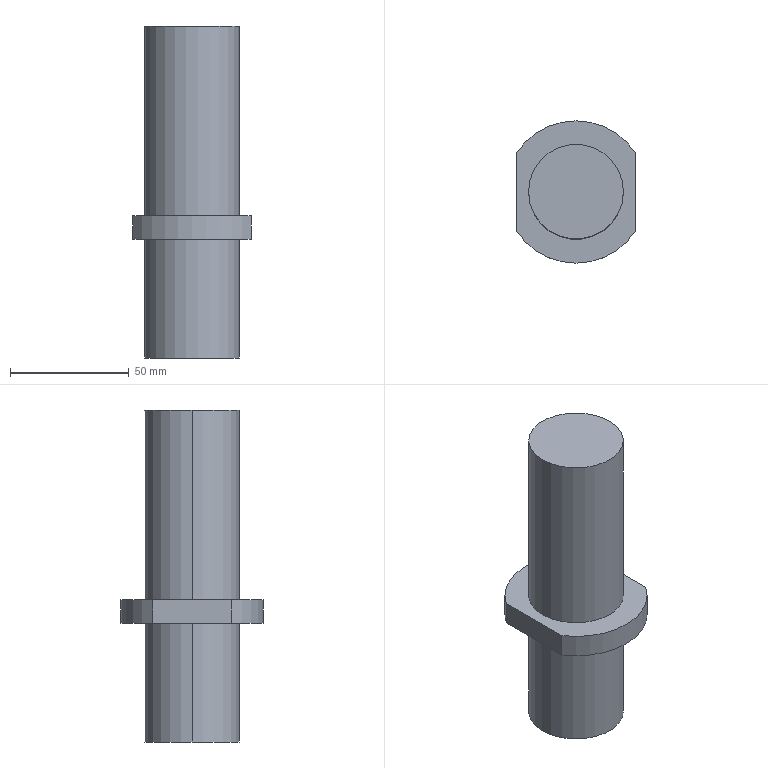Part | STEP file | Single sprocket shaft 1XG | 1 solid | 20 faces | box 50 x 60 x 140 mm | volume 188778 mm3 | cylinder 10 | plane 6 | cone 4 | commonest cylinder face diameters 5 x4 40 x4 60 x2
STEP:
#1=CARTESIAN_POINT('',(0.,0.,0.));
#2=DIRECTION('',(0.,0.,1.));
#3=DIRECTION('',(1.,0.,0.));
#4=AXIS2_PLACEMENT_3D('',#1,#2,#3);
#5=CARTESIAN_POINT('',(7.5,0.,15.));
#6=VERTEX_POINT('',#5);
#7=CARTESIAN_POINT('',(7.5,0.,0.));
#8=VERTEX_POINT('',#7);
#9=CARTESIAN_POINT('',(7.5,0.,0.));
#10=DIRECTION('',(0.,0.,-1.));
#11=VECTOR('',#10,1.);
#12=LINE('',#9,#11);
#13=CARTESIAN_POINT('',(10.,0.,0.));
#14=DIRECTION('',(0.,0.,-1.));
#15=DIRECTION('',(-1.,0.,0.));
#16=AXIS2_PLACEMENT_3D('',#13,#14,#15);
#17=CYLINDRICAL_SURFACE('',#16,2.5);
#18=CARTESIAN_POINT('',(6.283,0.));
#19=DIRECTION('',(0.,1.));
#20=VECTOR('',#19,1.);
#21=LINE('',#18,#20);
#22=(GEOMETRIC_REPRESENTATION_CONTEXT(2)PARAMETRIC_REPRESENTATION_CONTEXT()REPRESENTATION_CONTEXT('',''));
#23=DEFINITIONAL_REPRESENTATION('',(#21),#22);
#24=PCURVE('',#17,#23);
#25=CARTESIAN_POINT('',(10.,0.,0.));
#26=DIRECTION('',(0.,0.,-1.));
#27=DIRECTION('',(-1.,0.,0.));
#28=AXIS2_PLACEMENT_3D('',#25,#26,#27);
#29=CYLINDRICAL_SURFACE('',#28,2.5);
#30=CARTESIAN_POINT('',(0.,0.));
#31=DIRECTION('',(0.,1.));
#32=VECTOR('',#31,1.);
#33=LINE('',#30,#32);
#34=(GEOMETRIC_REPRESENTATION_CONTEXT(2)PARAMETRIC_REPRESENTATION_CONTEXT()REPRESENTATION_CONTEXT('',''));
#35=DEFINITIONAL_REPRESENTATION('',(#33),#34);
#36=PCURVE('',#29,#35);
#37=SURFACE_CURVE('',#12,(#24,#36),.PCURVE_S1.);
#38=EDGE_CURVE('',#6,#8,#37,.T.);
#39=ORIENTED_EDGE('',*,*,#38,.T.);
#40=CARTESIAN_POINT('',(12.5,0.,0.));
#41=VERTEX_POINT('',#40);
#42=CARTESIAN_POINT('',(10.,0.,0.));
#43=DIRECTION('',(0.,0.,-1.));
#44=DIRECTION('',(-1.,0.,0.));
#45=AXIS2_PLACEMENT_3D('',#42,#43,#44);
#46=CIRCLE('',#45,2.5);
#47=CARTESIAN_POINT('',(0.,0.));
#48=DIRECTION('',(1.,0.));
#49=VECTOR('',#48,1.);
#50=LINE('',#47,#49);
#51=(GEOMETRIC_REPRESENTATION_CONTEXT(2)PARAMETRIC_REPRESENTATION_CONTEXT()REPRESENTATION_CONTEXT('',''));
#52=DEFINITIONAL_REPRESENTATION('',(#50),#51);
#53=PCURVE('',#17,#52);
#54=CARTESIAN_POINT('',(0.,0.,0.));
#55=DIRECTION('',(0.,0.,1.));
#56=DIRECTION('',(1.,0.,0.));
#57=AXIS2_PLACEMENT_3D('',#54,#55,#56);
#58=PLANE('',#57);
#59=CARTESIAN_POINT('',(7.5,0.));
#60=CARTESIAN_POINT('',(7.5,4.33));
#61=CARTESIAN_POINT('',(11.25,2.165));
#62=CARTESIAN_POINT('',(15.,0.));
#63=CARTESIAN_POINT('',(11.25,-2.165));
#64=CARTESIAN_POINT('',(7.5,-4.33));
#65=CARTESIAN_POINT('',(7.5,0.));
#66=(BOUNDED_CURVE()B_SPLINE_CURVE(2,(#59,#60,#61,#62,#63,#64,#65),.UNSPECIFIED.,.T.,.F.)B_SPLINE_CURVE_WITH_KNOTS((1,2,2,2,2,1),(-2.094,0.,2.094,4.189,6.283,8.378),.UNSPECIFIED.)CURVE()GEOMETRIC_REPRESENTATION_ITEM()RATIONAL_B_SPLINE_CURVE((1.,0.5,1.,0.5,1.,0.5,1.))REPRESENTATION_ITEM(''));
#67=(GEOMETRIC_REPRESENTATION_CONTEXT(2)PARAMETRIC_REPRESENTATION_CONTEXT()REPRESENTATION_CONTEXT('',''));
#68=DEFINITIONAL_REPRESENTATION('',(#66),#67);
#69=PCURVE('',#58,#68);
#70=SURFACE_CURVE('',#46,(#53,#69),.PCURVE_S1.);
#71=EDGE_CURVE('',#41,#8,#70,.T.);
#72=ORIENTED_EDGE('',*,*,#71,.F.);
#73=CARTESIAN_POINT('',(12.5,0.,15.));
#74=VERTEX_POINT('',#73);
#75=CARTESIAN_POINT('',(12.5,0.,0.));
#76=DIRECTION('',(0.,0.,-1.));
#77=VECTOR('',#76,1.);
#78=LINE('',#75,#77);
#79=CARTESIAN_POINT('',(3.142,0.));
#80=DIRECTION('',(0.,1.));
#81=VECTOR('',#80,1.);
#82=LINE('',#79,#81);
#83=(GEOMETRIC_REPRESENTATION_CONTEXT(2)PARAMETRIC_REPRESENTATION_CONTEXT()REPRESENTATION_CONTEXT('',''));
#84=DEFINITIONAL_REPRESENTATION('',(#82),#83);
#85=PCURVE('',#17,#84);
#86=CARTESIAN_POINT('',(3.142,0.));
#87=DIRECTION('',(0.,1.));
#88=VECTOR('',#87,1.);
#89=LINE('',#86,#88);
#90=(GEOMETRIC_REPRESENTATION_CONTEXT(2)PARAMETRIC_REPRESENTATION_CONTEXT()REPRESENTATION_CONTEXT('',''));
#91=DEFINITIONAL_REPRESENTATION('',(#89),#90);
#92=PCURVE('',#29,#91);
#93=SURFACE_CURVE('',#78,(#85,#92),.PCURVE_S1.);
#94=EDGE_CURVE('',#74,#41,#93,.T.);
#95=ORIENTED_EDGE('',*,*,#94,.F.);
#96=CARTESIAN_POINT('',(10.,0.,15.));
#97=DIRECTION('',(0.,0.,-1.));
#98=DIRECTION('',(-1.,0.,0.));
#99=AXIS2_PLACEMENT_3D('',#96,#97,#98);
#100=CIRCLE('',#99,2.5);
#101=CARTESIAN_POINT('',(0.,-15.));
#102=DIRECTION('',(1.,0.));
#103=VECTOR('',#102,1.);
#104=LINE('',#101,#103);
#105=(GEOMETRIC_REPRESENTATION_CONTEXT(2)PARAMETRIC_REPRESENTATION_CONTEXT()REPRESENTATION_CONTEXT('',''));
#106=DEFINITIONAL_REPRESENTATION('',(#104),#105);
#107=PCURVE('',#17,#106);
#108=CARTESIAN_POINT('',(10.,0.,15.));
#109=DIRECTION('',(0.,0.,-1.));
#110=DIRECTION('',(-1.,0.,0.));
#111=AXIS2_PLACEMENT_3D('',#108,#109,#110);
#112=CONICAL_SURFACE('',#111,2.5,1.03);
#113=CARTESIAN_POINT('',(0.,0.));
#114=DIRECTION('',(1.,0.));
#115=VECTOR('',#114,1.);
#116=LINE('',#113,#115);
#117=(GEOMETRIC_REPRESENTATION_CONTEXT(2)PARAMETRIC_REPRESENTATION_CONTEXT()REPRESENTATION_CONTEXT('',''));
#118=DEFINITIONAL_REPRESENTATION('',(#116),#117);
#119=PCURVE('',#112,#118);
#120=SURFACE_CURVE('',#100,(#107,#119),.PCURVE_S1.);
#121=EDGE_CURVE('',#74,#6,#120,.T.);
#122=ORIENTED_EDGE('',*,*,#121,.T.);
#123=EDGE_LOOP('',(#39,#72,#95,#122));
#124=FACE_BOUND('',#123,.F.);
#125=ADVANCED_FACE('',(#124),#17,.F.);
#126=ORIENTED_EDGE('',*,*,#121,.F.);
#127=CARTESIAN_POINT('',(10.,0.,16.502));
#128=VERTEX_POINT('',#127);
#129=CARTESIAN_POINT('',(12.5,0.,15.));
#130=DIRECTION('',(0.8572,0.,-0.515));
#131=VECTOR('',#130,1.);
#132=LINE('',#129,#131);
#133=CARTESIAN_POINT('',(3.142,0.));
#134=DIRECTION('',(0.,1.));
#135=VECTOR('',#134,1.);
#136=LINE('',#133,#135);
#137=(GEOMETRIC_REPRESENTATION_CONTEXT(2)PARAMETRIC_REPRESENTATION_CONTEXT()REPRESENTATION_CONTEXT('',''));
#138=DEFINITIONAL_REPRESENTATION('',(#136),#137);
#139=PCURVE('',#112,#138);
#140=CARTESIAN_POINT('',(10.,0.,15.));
#141=DIRECTION('',(0.,0.,-1.));
#142=DIRECTION('',(-1.,0.,0.));
#143=AXIS2_PLACEMENT_3D('',#140,#141,#142);
#144=CONICAL_SURFACE('',#143,2.5,1.03);
#145=CARTESIAN_POINT('',(3.142,0.));
#146=DIRECTION('',(0.,1.));
#147=VECTOR('',#146,1.);
#148=LINE('',#145,#147);
#149=(GEOMETRIC_REPRESENTATION_CONTEXT(2)PARAMETRIC_REPRESENTATION_CONTEXT()REPRESENTATION_CONTEXT('',''));
#150=DEFINITIONAL_REPRESENTATION('',(#148),#149);
#151=PCURVE('',#144,#150);
#152=SURFACE_CURVE('',#132,(#139,#151),.PCURVE_S1.);
#153=EDGE_CURVE('',#128,#74,#152,.T.);
#154=ORIENTED_EDGE('',*,*,#153,.F.);
#155=CARTESIAN_POINT('',(7.5,0.,15.));
#156=DIRECTION('',(-0.8572,0.,-0.515));
#157=VECTOR('',#156,1.);
#158=LINE('',#155,#157);
#159=CARTESIAN_POINT('',(6.283,0.));
#160=DIRECTION('',(0.,1.));
#161=VECTOR('',#160,1.);
#162=LINE('',#159,#161);
#163=(GEOMETRIC_REPRESENTATION_CONTEXT(2)PARAMETRIC_REPRESENTATION_CONTEXT()REPRESENTATION_CONTEXT('',''));
#164=DEFINITIONAL_REPRESENTATION('',(#162),#163);
#165=PCURVE('',#112,#164);
#166=CARTESIAN_POINT('',(0.,0.));
#167=DIRECTION('',(0.,1.));
#168=VECTOR('',#167,1.);
#169=LINE('',#166,#168);
#170=(GEOMETRIC_REPRESENTATION_CONTEXT(2)PARAMETRIC_REPRESENTATION_CONTEXT()REPRESENTATION_CONTEXT('',''));
#171=DEFINITIONAL_REPRESENTATION('',(#169),#170);
#172=PCURVE('',#144,#171);
#173=SURFACE_CURVE('',#158,(#165,#172),.PCURVE_S1.);
#174=EDGE_CURVE('',#128,#6,#173,.T.);
#175=ORIENTED_EDGE('',*,*,#174,.T.);
#176=EDGE_LOOP('',(#126,#154,#175));
#177=FACE_BOUND('',#176,.F.);
#178=ADVANCED_FACE('',(#177),#112,.F.);
#179=CARTESIAN_POINT('',(-12.5,0.,15.));
#180=VERTEX_POINT('',#179);
#181=CARTESIAN_POINT('',(-12.5,0.,0.));
#182=VERTEX_POINT('',#181);
#183=CARTESIAN_POINT('',(-12.5,0.,0.));
#184=DIRECTION('',(0.,0.,-1.));
#185=VECTOR('',#184,1.);
#186=LINE('',#183,#185);
#187=CARTESIAN_POINT('',(-10.,0.,0.));
#188=DIRECTION('',(0.,0.,-1.));
#189=DIRECTION('',(-1.,0.,0.));
#190=AXIS2_PLACEMENT_3D('',#187,#188,#189);
#191=CYLINDRICAL_SURFACE('',#190,2.5);
#192=CARTESIAN_POINT('',(6.283,0.));
#193=DIRECTION('',(0.,1.));
#194=VECTOR('',#193,1.);
#195=LINE('',#192,#194);
#196=(GEOMETRIC_REPRESENTATION_CONTEXT(2)PARAMETRIC_REPRESENTATION_CONTEXT()REPRESENTATION_CONTEXT('',''));
#197=DEFINITIONAL_REPRESENTATION('',(#195),#196);
#198=PCURVE('',#191,#197);
#199=CARTESIAN_POINT('',(-10.,0.,0.));
#200=DIRECTION('',(0.,0.,-1.));
#201=DIRECTION('',(-1.,0.,0.));
#202=AXIS2_PLACEMENT_3D('',#199,#200,#201);
#203=CYLINDRICAL_SURFACE('',#202,2.5);
#204=CARTESIAN_POINT('',(0.,0.));
#205=DIRECTION('',(0.,1.));
#206=VECTOR('',#205,1.);
#207=LINE('',#204,#206);
#208=(GEOMETRIC_REPRESENTATION_CONTEXT(2)PARAMETRIC_REPRESENTATION_CONTEXT()REPRESENTATION_CONTEXT('',''));
#209=DEFINITIONAL_REPRESENTATION('',(#207),#208);
#210=PCURVE('',#203,#209);
#211=SURFACE_CURVE('',#186,(#198,#210),.PCURVE_S1.);
#212=EDGE_CURVE('',#180,#182,#211,.T.);
#213=ORIENTED_EDGE('',*,*,#212,.T.);
#214=CARTESIAN_POINT('',(-7.5,0.,0.));
#215=VERTEX_POINT('',#214);
#216=CARTESIAN_POINT('',(-10.,0.,0.));
#217=DIRECTION('',(0.,0.,-1.));
#218=DIRECTION('',(-1.,0.,0.));
#219=AXIS2_PLACEMENT_3D('',#216,#217,#218);
#220=CIRCLE('',#219,2.5);
#221=CARTESIAN_POINT('',(0.,0.));
#222=DIRECTION('',(1.,0.));
#223=VECTOR('',#222,1.);
#224=LINE('',#221,#223);
#225=(GEOMETRIC_REPRESENTATION_CONTEXT(2)PARAMETRIC_REPRESENTATION_CONTEXT()REPRESENTATION_CONTEXT('',''));
#226=DEFINITIONAL_REPRESENTATION('',(#224),#225);
#227=PCURVE('',#191,#226);
#228=CARTESIAN_POINT('',(-12.5,0.));
#229=CARTESIAN_POINT('',(-12.5,4.33));
#230=CARTESIAN_POINT('',(-8.75,2.165));
#231=CARTESIAN_POINT('',(-5.,0.));
#232=CARTESIAN_POINT('',(-8.75,-2.165));
#233=CARTESIAN_POINT('',(-12.5,-4.33));
#234=CARTESIAN_POINT('',(-12.5,0.));
#235=(BOUNDED_CURVE()B_SPLINE_CURVE(2,(#228,#229,#230,#231,#232,#233,#234),.UNSPECIFIED.,.T.,.F.)B_SPLINE_CURVE_WITH_KNOTS((1,2,2,2,2,1),(-2.094,0.,2.094,4.189,6.283,8.378),.UNSPECIFIED.)CURVE()GEOMETRIC_REPRESENTATION_ITEM()RATIONAL_B_SPLINE_CURVE((1.,0.5,1.,0.5,1.,0.5,1.))REPRESENTATION_ITEM(''));
#236=(GEOMETRIC_REPRESENTATION_CONTEXT(2)PARAMETRIC_REPRESENTATION_CONTEXT()REPRESENTATION_CONTEXT('',''));
#237=DEFINITIONAL_REPRESENTATION('',(#235),#236);
#238=PCURVE('',#58,#237);
#239=SURFACE_CURVE('',#220,(#227,#238),.PCURVE_S1.);
#240=EDGE_CURVE('',#215,#182,#239,.T.);
#241=ORIENTED_EDGE('',*,*,#240,.F.);
#242=CARTESIAN_POINT('',(-7.5,0.,15.));
#243=VERTEX_POINT('',#242);
#244=CARTESIAN_POINT('',(-7.5,0.,0.));
#245=DIRECTION('',(0.,0.,-1.));
#246=VECTOR('',#245,1.);
#247=LINE('',#244,#246);
#248=CARTESIAN_POINT('',(3.142,0.));
#249=DIRECTION('',(0.,1.));
#250=VECTOR('',#249,1.);
#251=LINE('',#248,#250);
#252=(GEOMETRIC_REPRESENTATION_CONTEXT(2)PARAMETRIC_REPRESENTATION_CONTEXT()REPRESENTATION_CONTEXT('',''));
#253=DEFINITIONAL_REPRESENTATION('',(#251),#252);
#254=PCURVE('',#191,#253);
#255=CARTESIAN_POINT('',(3.142,0.));
#256=DIRECTION('',(0.,1.));
#257=VECTOR('',#256,1.);
#258=LINE('',#255,#257);
#259=(GEOMETRIC_REPRESENTATION_CONTEXT(2)PARAMETRIC_REPRESENTATION_CONTEXT()REPRESENTATION_CONTEXT('',''));
#260=DEFINITIONAL_REPRESENTATION('',(#258),#259);
#261=PCURVE('',#203,#260);
#262=SURFACE_CURVE('',#247,(#254,#261),.PCURVE_S1.);
#263=EDGE_CURVE('',#243,#215,#262,.T.);
#264=ORIENTED_EDGE('',*,*,#263,.F.);
#265=CARTESIAN_POINT('',(-10.,0.,15.));
#266=DIRECTION('',(0.,0.,-1.));
#267=DIRECTION('',(-1.,0.,0.));
#268=AXIS2_PLACEMENT_3D('',#265,#266,#267);
#269=CIRCLE('',#268,2.5);
#270=CARTESIAN_POINT('',(0.,-15.));
#271=DIRECTION('',(1.,0.));
#272=VECTOR('',#271,1.);
#273=LINE('',#270,#272);
#274=(GEOMETRIC_REPRESENTATION_CONTEXT(2)PARAMETRIC_REPRESENTATION_CONTEXT()REPRESENTATION_CONTEXT('',''));
#275=DEFINITIONAL_REPRESENTATION('',(#273),#274);
#276=PCURVE('',#191,#275);
#277=CARTESIAN_POINT('',(-10.,0.,15.));
#278=DIRECTION('',(0.,0.,-1.));
#279=DIRECTION('',(-1.,0.,0.));
#280=AXIS2_PLACEMENT_3D('',#277,#278,#279);
#281=CONICAL_SURFACE('',#280,2.5,1.03);
#282=CARTESIAN_POINT('',(0.,0.));
#283=DIRECTION('',(1.,0.));
#284=VECTOR('',#283,1.);
#285=LINE('',#282,#284);
#286=(GEOMETRIC_REPRESENTATION_CONTEXT(2)PARAMETRIC_REPRESENTATION_CONTEXT()REPRESENTATION_CONTEXT('',''));
#287=DEFINITIONAL_REPRESENTATION('',(#285),#286);
#288=PCURVE('',#281,#287);
#289=SURFACE_CURVE('',#269,(#276,#288),.PCURVE_S1.);
#290=EDGE_CURVE('',#243,#180,#289,.T.);
#291=ORIENTED_EDGE('',*,*,#290,.T.);
#292=EDGE_LOOP('',(#213,#241,#264,#291));
#293=FACE_BOUND('',#292,.F.);
#294=ADVANCED_FACE('',(#293),#191,.F.);
#295=ORIENTED_EDGE('',*,*,#290,.F.);
#296=CARTESIAN_POINT('',(-10.,0.,16.502));
#297=VERTEX_POINT('',#296);
#298=CARTESIAN_POINT('',(-7.5,0.,15.));
#299=DIRECTION('',(0.8572,0.,-0.515));
#300=VECTOR('',#299,1.);
#301=LINE('',#298,#300);
#302=CARTESIAN_POINT('',(3.142,0.));
#303=DIRECTION('',(0.,1.));
#304=VECTOR('',#303,1.);
#305=LINE('',#302,#304);
#306=(GEOMETRIC_REPRESENTATION_CONTEXT(2)PARAMETRIC_REPRESENTATION_CONTEXT()REPRESENTATION_CONTEXT('',''));
#307=DEFINITIONAL_REPRESENTATION('',(#305),#306);
#308=PCURVE('',#281,#307);
#309=CARTESIAN_POINT('',(-10.,0.,15.));
#310=DIRECTION('',(0.,0.,-1.));
#311=DIRECTION('',(-1.,0.,0.));
#312=AXIS2_PLACEMENT_3D('',#309,#310,#311);
#313=CONICAL_SURFACE('',#312,2.5,1.03);
#314=CARTESIAN_POINT('',(3.142,0.));
#315=DIRECTION('',(0.,1.));
#316=VECTOR('',#315,1.);
#317=LINE('',#314,#316);
#318=(GEOMETRIC_REPRESENTATION_CONTEXT(2)PARAMETRIC_REPRESENTATION_CONTEXT()REPRESENTATION_CONTEXT('',''));
#319=DEFINITIONAL_REPRESENTATION('',(#317),#318);
#320=PCURVE('',#313,#319);
#321=SURFACE_CURVE('',#301,(#308,#320),.PCURVE_S1.);
#322=EDGE_CURVE('',#297,#243,#321,.T.);
#323=ORIENTED_EDGE('',*,*,#322,.F.);
#324=CARTESIAN_POINT('',(-12.5,0.,15.));
#325=DIRECTION('',(-0.8572,0.,-0.515));
#326=VECTOR('',#325,1.);
#327=LINE('',#324,#326);
#328=CARTESIAN_POINT('',(6.283,0.));
#329=DIRECTION('',(0.,1.));
#330=VECTOR('',#329,1.);
#331=LINE('',#328,#330);
#332=(GEOMETRIC_REPRESENTATION_CONTEXT(2)PARAMETRIC_REPRESENTATION_CONTEXT()REPRESENTATION_CONTEXT('',''));
#333=DEFINITIONAL_REPRESENTATION('',(#331),#332);
#334=PCURVE('',#281,#333);
#335=CARTESIAN_POINT('',(0.,0.));
#336=DIRECTION('',(0.,1.));
#337=VECTOR('',#336,1.);
#338=LINE('',#335,#337);
#339=(GEOMETRIC_REPRESENTATION_CONTEXT(2)PARAMETRIC_REPRESENTATION_CONTEXT()REPRESENTATION_CONTEXT('',''));
#340=DEFINITIONAL_REPRESENTATION('',(#338),#339);
#341=PCURVE('',#313,#340);
#342=SURFACE_CURVE('',#327,(#334,#341),.PCURVE_S1.);
#343=EDGE_CURVE('',#297,#180,#342,.T.);
#344=ORIENTED_EDGE('',*,*,#343,.T.);
#345=EDGE_LOOP('',(#295,#323,#344));
#346=FACE_BOUND('',#345,.F.);
#347=ADVANCED_FACE('',(#346),#281,.F.);
#348=CARTESIAN_POINT('',(20.,0.,140.));
#349=VERTEX_POINT('',#348);
#350=CARTESIAN_POINT('',(-20.,0.,140.));
#351=VERTEX_POINT('',#350);
#352=CARTESIAN_POINT('',(0.,0.,140.));
#353=DIRECTION('',(0.,0.,1.));
#354=DIRECTION('',(1.,0.,0.));
#355=AXIS2_PLACEMENT_3D('',#352,#353,#354);
#356=CIRCLE('',#355,20.);
#357=CARTESIAN_POINT('',(0.,0.,140.));
#358=DIRECTION('',(0.,0.,-1.));
#359=DIRECTION('',(-1.,0.,0.));
#360=AXIS2_PLACEMENT_3D('',#357,#358,#359);
#361=CYLINDRICAL_SURFACE('',#360,20.);
#362=CARTESIAN_POINT('',(3.142,0.));
#363=DIRECTION('',(-1.,0.));
#364=VECTOR('',#363,1.);
#365=LINE('',#362,#364);
#366=(GEOMETRIC_REPRESENTATION_CONTEXT(2)PARAMETRIC_REPRESENTATION_CONTEXT()REPRESENTATION_CONTEXT('',''));
#367=DEFINITIONAL_REPRESENTATION('',(#365),#366);
#368=PCURVE('',#361,#367);
#369=CARTESIAN_POINT('',(0.,0.,140.));
#370=DIRECTION('',(0.,0.,1.));
#371=DIRECTION('',(1.,0.,0.));
#372=AXIS2_PLACEMENT_3D('',#369,#370,#371);
#373=PLANE('',#372);
#374=CARTESIAN_POINT('',(0.,0.));
#375=DIRECTION('',(1.,0.));
#376=AXIS2_PLACEMENT_2D('',#374,#375);
#377=CIRCLE('',#376,20.);
#378=(GEOMETRIC_REPRESENTATION_CONTEXT(2)PARAMETRIC_REPRESENTATION_CONTEXT()REPRESENTATION_CONTEXT('',''));
#379=DEFINITIONAL_REPRESENTATION('',(#377),#378);
#380=PCURVE('',#373,#379);
#381=SURFACE_CURVE('',#356,(#368,#380),.PCURVE_S1.);
#382=EDGE_CURVE('',#349,#351,#381,.T.);
#383=ORIENTED_EDGE('',*,*,#382,.F.);
#384=CARTESIAN_POINT('',(20.,0.,60.));
#385=VERTEX_POINT('',#384);
#386=CARTESIAN_POINT('',(20.,0.,140.));
#387=DIRECTION('',(0.,0.,-1.));
#388=VECTOR('',#387,1.);
#389=LINE('',#386,#388);
#390=CARTESIAN_POINT('',(3.142,0.));
#391=DIRECTION('',(0.,1.));
#392=VECTOR('',#391,1.);
#393=LINE('',#390,#392);
#394=(GEOMETRIC_REPRESENTATION_CONTEXT(2)PARAMETRIC_REPRESENTATION_CONTEXT()REPRESENTATION_CONTEXT('',''));
#395=DEFINITIONAL_REPRESENTATION('',(#393),#394);
#396=PCURVE('',#361,#395);
#397=CARTESIAN_POINT('',(0.,0.,140.));
#398=DIRECTION('',(0.,0.,-1.));
#399=DIRECTION('',(-1.,0.,0.));
#400=AXIS2_PLACEMENT_3D('',#397,#398,#399);
#401=CYLINDRICAL_SURFACE('',#400,20.);
#402=CARTESIAN_POINT('',(3.142,0.));
#403=DIRECTION('',(0.,1.));
#404=VECTOR('',#403,1.);
#405=LINE('',#402,#404);
#406=(GEOMETRIC_REPRESENTATION_CONTEXT(2)PARAMETRIC_REPRESENTATION_CONTEXT()REPRESENTATION_CONTEXT('',''));
#407=DEFINITIONAL_REPRESENTATION('',(#405),#406);
#408=PCURVE('',#401,#407);
#409=SURFACE_CURVE('',#389,(#396,#408),.PCURVE_S1.);
#410=EDGE_CURVE('',#349,#385,#409,.T.);
#411=ORIENTED_EDGE('',*,*,#410,.T.);
#412=CARTESIAN_POINT('',(-20.,0.,60.));
#413=VERTEX_POINT('',#412);
#414=CARTESIAN_POINT('',(0.,0.,60.));
#415=DIRECTION('',(0.,0.,1.));
#416=DIRECTION('',(1.,0.,0.));
#417=AXIS2_PLACEMENT_3D('',#414,#415,#416);
#418=CIRCLE('',#417,20.);
#419=CARTESIAN_POINT('',(3.142,80.));
#420=DIRECTION('',(-1.,0.));
#421=VECTOR('',#420,1.);
#422=LINE('',#419,#421);
#423=(GEOMETRIC_REPRESENTATION_CONTEXT(2)PARAMETRIC_REPRESENTATION_CONTEXT()REPRESENTATION_CONTEXT('',''));
#424=DEFINITIONAL_REPRESENTATION('',(#422),#423);
#425=PCURVE('',#361,#424);
#426=CARTESIAN_POINT('',(0.,0.,60.));
#427=DIRECTION('',(0.,0.,1.));
#428=DIRECTION('',(1.,0.,0.));
#429=AXIS2_PLACEMENT_3D('',#426,#427,#428);
#430=PLANE('',#429);
#431=CARTESIAN_POINT('',(0.,0.));
#432=DIRECTION('',(1.,0.));
#433=AXIS2_PLACEMENT_2D('',#431,#432);
#434=CIRCLE('',#433,20.);
#435=(GEOMETRIC_REPRESENTATION_CONTEXT(2)PARAMETRIC_REPRESENTATION_CONTEXT()REPRESENTATION_CONTEXT('',''));
#436=DEFINITIONAL_REPRESENTATION('',(#434),#435);
#437=PCURVE('',#430,#436);
#438=SURFACE_CURVE('',#418,(#425,#437),.PCURVE_S1.);
#439=EDGE_CURVE('',#385,#413,#438,.T.);
#440=ORIENTED_EDGE('',*,*,#439,.T.);
#441=CARTESIAN_POINT('',(-20.,0.,140.));
#442=DIRECTION('',(0.,0.,-1.));
#443=VECTOR('',#442,1.);
#444=LINE('',#441,#443);
#445=CARTESIAN_POINT('',(0.,0.));
#446=DIRECTION('',(0.,1.));
#447=VECTOR('',#446,1.);
#448=LINE('',#445,#447);
#449=(GEOMETRIC_REPRESENTATION_CONTEXT(2)PARAMETRIC_REPRESENTATION_CONTEXT()REPRESENTATION_CONTEXT('',''));
#450=DEFINITIONAL_REPRESENTATION('',(#448),#449);
#451=PCURVE('',#361,#450);
#452=CARTESIAN_POINT('',(6.283,0.));
#453=DIRECTION('',(0.,1.));
#454=VECTOR('',#453,1.);
#455=LINE('',#452,#454);
#456=(GEOMETRIC_REPRESENTATION_CONTEXT(2)PARAMETRIC_REPRESENTATION_CONTEXT()REPRESENTATION_CONTEXT('',''));
#457=DEFINITIONAL_REPRESENTATION('',(#455),#456);
#458=PCURVE('',#401,#457);
#459=SURFACE_CURVE('',#444,(#451,#458),.PCURVE_S1.);
#460=EDGE_CURVE('',#351,#413,#459,.T.);
#461=ORIENTED_EDGE('',*,*,#460,.F.);
#462=EDGE_LOOP('',(#383,#411,#440,#461));
#463=FACE_BOUND('',#462,.T.);
#464=ADVANCED_FACE('',(#463),#361,.T.);
#465=CARTESIAN_POINT('',(20.,0.,50.));
#466=VERTEX_POINT('',#465);
#467=CARTESIAN_POINT('',(-20.,0.,50.));
#468=VERTEX_POINT('',#467);
#469=CARTESIAN_POINT('',(0.,0.,50.));
#470=DIRECTION('',(0.,0.,1.));
#471=DIRECTION('',(1.,0.,0.));
#472=AXIS2_PLACEMENT_3D('',#469,#470,#471);
#473=CIRCLE('',#472,20.);
#474=CARTESIAN_POINT('',(0.,0.,50.));
#475=DIRECTION('',(0.,0.,-1.));
#476=DIRECTION('',(-1.,0.,0.));
#477=AXIS2_PLACEMENT_3D('',#474,#475,#476);
#478=CYLINDRICAL_SURFACE('',#477,20.);
#479=CARTESIAN_POINT('',(3.142,0.));
#480=DIRECTION('',(-1.,0.));
#481=VECTOR('',#480,1.);
#482=LINE('',#479,#481);
#483=(GEOMETRIC_REPRESENTATION_CONTEXT(2)PARAMETRIC_REPRESENTATION_CONTEXT()REPRESENTATION_CONTEXT('',''));
#484=DEFINITIONAL_REPRESENTATION('',(#482),#483);
#485=PCURVE('',#478,#484);
#486=CARTESIAN_POINT('',(0.,0.,50.));
#487=DIRECTION('',(0.,0.,1.));
#488=DIRECTION('',(1.,0.,0.));
#489=AXIS2_PLACEMENT_3D('',#486,#487,#488);
#490=PLANE('',#489);
#491=CARTESIAN_POINT('',(0.,0.));
#492=DIRECTION('',(1.,0.));
#493=AXIS2_PLACEMENT_2D('',#491,#492);
#494=CIRCLE('',#493,20.);
#495=(GEOMETRIC_REPRESENTATION_CONTEXT(2)PARAMETRIC_REPRESENTATION_CONTEXT()REPRESENTATION_CONTEXT('',''));
#496=DEFINITIONAL_REPRESENTATION('',(#494),#495);
#497=PCURVE('',#490,#496);
#498=SURFACE_CURVE('',#473,(#485,#497),.PCURVE_S1.);
#499=EDGE_CURVE('',#466,#468,#498,.T.);
#500=ORIENTED_EDGE('',*,*,#499,.F.);
#501=CARTESIAN_POINT('',(20.,0.,0.));
#502=VERTEX_POINT('',#501);
#503=CARTESIAN_POINT('',(20.,0.,50.));
#504=DIRECTION('',(0.,0.,-1.));
#505=VECTOR('',#504,1.);
#506=LINE('',#503,#505);
#507=CARTESIAN_POINT('',(3.142,0.));
#508=DIRECTION('',(0.,1.));
#509=VECTOR('',#508,1.);
#510=LINE('',#507,#509);
#511=(GEOMETRIC_REPRESENTATION_CONTEXT(2)PARAMETRIC_REPRESENTATION_CONTEXT()REPRESENTATION_CONTEXT('',''));
#512=DEFINITIONAL_REPRESENTATION('',(#510),#511);
#513=PCURVE('',#478,#512);
#514=CARTESIAN_POINT('',(0.,0.,50.));
#515=DIRECTION('',(0.,0.,-1.));
#516=DIRECTION('',(-1.,0.,0.));
#517=AXIS2_PLACEMENT_3D('',#514,#515,#516);
#518=CYLINDRICAL_SURFACE('',#517,20.);
#519=CARTESIAN_POINT('',(3.142,0.));
#520=DIRECTION('',(0.,1.));
#521=VECTOR('',#520,1.);
#522=LINE('',#519,#521);
#523=(GEOMETRIC_REPRESENTATION_CONTEXT(2)PARAMETRIC_REPRESENTATION_CONTEXT()REPRESENTATION_CONTEXT('',''));
#524=DEFINITIONAL_REPRESENTATION('',(#522),#523);
#525=PCURVE('',#518,#524);
#526=SURFACE_CURVE('',#506,(#513,#525),.PCURVE_S1.);
#527=EDGE_CURVE('',#466,#502,#526,.T.);
#528=ORIENTED_EDGE('',*,*,#527,.T.);
#529=CARTESIAN_POINT('',(-20.,0.,0.));
#530=VERTEX_POINT('',#529);
#531=CARTESIAN_POINT('',(0.,0.,0.));
#532=DIRECTION('',(0.,0.,1.));
#533=DIRECTION('',(1.,0.,0.));
#534=AXIS2_PLACEMENT_3D('',#531,#532,#533);
#535=CIRCLE('',#534,20.);
#536=CARTESIAN_POINT('',(3.142,50.));
#537=DIRECTION('',(-1.,0.));
#538=VECTOR('',#537,1.);
#539=LINE('',#536,#538);
#540=(GEOMETRIC_REPRESENTATION_CONTEXT(2)PARAMETRIC_REPRESENTATION_CONTEXT()REPRESENTATION_CONTEXT('',''));
#541=DEFINITIONAL_REPRESENTATION('',(#539),#540);
#542=PCURVE('',#478,#541);
#543=CARTESIAN_POINT('',(0.,0.));
#544=DIRECTION('',(1.,0.));
#545=AXIS2_PLACEMENT_2D('',#543,#544);
#546=CIRCLE('',#545,20.);
#547=(GEOMETRIC_REPRESENTATION_CONTEXT(2)PARAMETRIC_REPRESENTATION_CONTEXT()REPRESENTATION_CONTEXT('',''));
#548=DEFINITIONAL_REPRESENTATION('',(#546),#547);
#549=PCURVE('',#58,#548);
#550=SURFACE_CURVE('',#535,(#542,#549),.PCURVE_S1.);
#551=EDGE_CURVE('',#502,#530,#550,.T.);
#552=ORIENTED_EDGE('',*,*,#551,.T.);
#553=CARTESIAN_POINT('',(-20.,0.,50.));
#554=DIRECTION('',(0.,0.,-1.));
#555=VECTOR('',#554,1.);
#556=LINE('',#553,#555);
#557=CARTESIAN_POINT('',(0.,0.));
#558=DIRECTION('',(0.,1.));
#559=VECTOR('',#558,1.);
#560=LINE('',#557,#559);
#561=(GEOMETRIC_REPRESENTATION_CONTEXT(2)PARAMETRIC_REPRESENTATION_CONTEXT()REPRESENTATION_CONTEXT('',''));
#562=DEFINITIONAL_REPRESENTATION('',(#560),#561);
#563=PCURVE('',#478,#562);
#564=CARTESIAN_POINT('',(6.283,0.));
#565=DIRECTION('',(0.,1.));
#566=VECTOR('',#565,1.);
#567=LINE('',#564,#566);
#568=(GEOMETRIC_REPRESENTATION_CONTEXT(2)PARAMETRIC_REPRESENTATION_CONTEXT()REPRESENTATION_CONTEXT('',''));
#569=DEFINITIONAL_REPRESENTATION('',(#567),#568);
#570=PCURVE('',#518,#569);
#571=SURFACE_CURVE('',#556,(#563,#570),.PCURVE_S1.);
#572=EDGE_CURVE('',#468,#530,#571,.T.);
#573=ORIENTED_EDGE('',*,*,#572,.F.);
#574=EDGE_LOOP('',(#500,#528,#552,#573));
#575=FACE_BOUND('',#574,.T.);
#576=ADVANCED_FACE('',(#575),#478,.T.);
#577=CARTESIAN_POINT('',(-25.,-16.583,60.));
#578=VERTEX_POINT('',#577);
#579=CARTESIAN_POINT('',(25.,-16.583,60.));
#580=VERTEX_POINT('',#579);
#581=CARTESIAN_POINT('',(0.,0.,60.));
#582=DIRECTION('',(0.,0.,1.));
#583=DIRECTION('',(1.,0.,0.));
#584=AXIS2_PLACEMENT_3D('',#581,#582,#583);
#585=CIRCLE('',#584,30.);
#586=CARTESIAN_POINT('',(0.,0.));
#587=DIRECTION('',(1.,0.));
#588=AXIS2_PLACEMENT_2D('',#586,#587);
#589=CIRCLE('',#588,30.);
#590=(GEOMETRIC_REPRESENTATION_CONTEXT(2)PARAMETRIC_REPRESENTATION_CONTEXT()REPRESENTATION_CONTEXT('',''));
#591=DEFINITIONAL_REPRESENTATION('',(#589),#590);
#592=PCURVE('',#430,#591);
#593=CARTESIAN_POINT('',(0.,0.,60.));
#594=DIRECTION('',(0.,0.,-1.));
#595=DIRECTION('',(-1.,0.,0.));
#596=AXIS2_PLACEMENT_3D('',#593,#594,#595);
#597=CYLINDRICAL_SURFACE('',#596,30.);
#598=CARTESIAN_POINT('',(9.425,0.));
#599=DIRECTION('',(-1.,0.));
#600=VECTOR('',#599,1.);
#601=LINE('',#598,#600);
#602=(GEOMETRIC_REPRESENTATION_CONTEXT(2)PARAMETRIC_REPRESENTATION_CONTEXT()REPRESENTATION_CONTEXT('',''));
#603=DEFINITIONAL_REPRESENTATION('',(#601),#602);
#604=PCURVE('',#597,#603);
#605=SURFACE_CURVE('',#585,(#592,#604),.PCURVE_S1.);
#606=EDGE_CURVE('',#578,#580,#605,.T.);
#607=ORIENTED_EDGE('',*,*,#606,.T.);
#608=CARTESIAN_POINT('',(25.,16.583,60.));
#609=VERTEX_POINT('',#608);
#610=CARTESIAN_POINT('',(25.,16.583,60.));
#611=DIRECTION('',(0.,1.,0.));
#612=VECTOR('',#611,1.);
#613=LINE('',#610,#612);
#614=CARTESIAN_POINT('',(25.,16.583));
#615=DIRECTION('',(0.,1.));
#616=VECTOR('',#615,1.);
#617=LINE('',#614,#616);
#618=(GEOMETRIC_REPRESENTATION_CONTEXT(2)PARAMETRIC_REPRESENTATION_CONTEXT()REPRESENTATION_CONTEXT('',''));
#619=DEFINITIONAL_REPRESENTATION('',(#617),#618);
#620=PCURVE('',#430,#619);
#621=CARTESIAN_POINT('',(25.,16.583,60.));
#622=DIRECTION('',(-1.,0.,0.));
#623=DIRECTION('',(0.,0.,1.));
#624=AXIS2_PLACEMENT_3D('',#621,#622,#623);
#625=PLANE('',#624);
#626=CARTESIAN_POINT('',(0.,0.));
#627=DIRECTION('',(0.,1.));
#628=VECTOR('',#627,1.);
#629=LINE('',#626,#628);
#630=(GEOMETRIC_REPRESENTATION_CONTEXT(2)PARAMETRIC_REPRESENTATION_CONTEXT()REPRESENTATION_CONTEXT('',''));
#631=DEFINITIONAL_REPRESENTATION('',(#629),#630);
#632=PCURVE('',#625,#631);
#633=SURFACE_CURVE('',#613,(#620,#632),.PCURVE_S1.);
#634=EDGE_CURVE('',#580,#609,#633,.T.);
#635=ORIENTED_EDGE('',*,*,#634,.T.);
#636=CARTESIAN_POINT('',(-25.,16.583,60.));
#637=VERTEX_POINT('',#636);
#638=CARTESIAN_POINT('',(0.,0.,60.));
#639=DIRECTION('',(0.,0.,1.));
#640=DIRECTION('',(1.,0.,0.));
#641=AXIS2_PLACEMENT_3D('',#638,#639,#640);
#642=CIRCLE('',#641,30.);
#643=CARTESIAN_POINT('',(0.,0.));
#644=DIRECTION('',(1.,0.));
#645=AXIS2_PLACEMENT_2D('',#643,#644);
#646=CIRCLE('',#645,30.);
#647=(GEOMETRIC_REPRESENTATION_CONTEXT(2)PARAMETRIC_REPRESENTATION_CONTEXT()REPRESENTATION_CONTEXT('',''));
#648=DEFINITIONAL_REPRESENTATION('',(#646),#647);
#649=PCURVE('',#430,#648);
#650=CARTESIAN_POINT('',(0.,0.,60.));
#651=DIRECTION('',(0.,0.,-1.));
#652=DIRECTION('',(-1.,0.,0.));
#653=AXIS2_PLACEMENT_3D('',#650,#651,#652);
#654=CYLINDRICAL_SURFACE('',#653,30.);
#655=CARTESIAN_POINT('',(3.142,0.));
#656=DIRECTION('',(-1.,0.));
#657=VECTOR('',#656,1.);
#658=LINE('',#655,#657);
#659=(GEOMETRIC_REPRESENTATION_CONTEXT(2)PARAMETRIC_REPRESENTATION_CONTEXT()REPRESENTATION_CONTEXT('',''));
#660=DEFINITIONAL_REPRESENTATION('',(#658),#659);
#661=PCURVE('',#654,#660);
#662=SURFACE_CURVE('',#642,(#649,#661),.PCURVE_S1.);
#663=EDGE_CURVE('',#609,#637,#662,.T.);
#664=ORIENTED_EDGE('',*,*,#663,.T.);
#665=CARTESIAN_POINT('',(-25.,16.583,60.));
#666=DIRECTION('',(0.,-1.,0.));
#667=VECTOR('',#666,1.);
#668=LINE('',#665,#667);
#669=CARTESIAN_POINT('',(-25.,16.583));
#670=DIRECTION('',(0.,-1.));
#671=VECTOR('',#670,1.);
#672=LINE('',#669,#671);
#673=(GEOMETRIC_REPRESENTATION_CONTEXT(2)PARAMETRIC_REPRESENTATION_CONTEXT()REPRESENTATION_CONTEXT('',''));
#674=DEFINITIONAL_REPRESENTATION('',(#672),#673);
#675=PCURVE('',#430,#674);
#676=CARTESIAN_POINT('',(-25.,16.583,60.));
#677=DIRECTION('',(1.,0.,0.));
#678=DIRECTION('',(0.,0.,-1.));
#679=AXIS2_PLACEMENT_3D('',#676,#677,#678);
#680=PLANE('',#679);
#681=CARTESIAN_POINT('',(0.,0.));
#682=DIRECTION('',(0.,-1.));
#683=VECTOR('',#682,1.);
#684=LINE('',#681,#683);
#685=(GEOMETRIC_REPRESENTATION_CONTEXT(2)PARAMETRIC_REPRESENTATION_CONTEXT()REPRESENTATION_CONTEXT('',''));
#686=DEFINITIONAL_REPRESENTATION('',(#684),#685);
#687=PCURVE('',#680,#686);
#688=SURFACE_CURVE('',#668,(#675,#687),.PCURVE_S1.);
#689=EDGE_CURVE('',#637,#578,#688,.T.);
#690=ORIENTED_EDGE('',*,*,#689,.T.);
#691=EDGE_LOOP('',(#607,#635,#664,#690));
#692=FACE_BOUND('',#691,.T.);
#693=CARTESIAN_POINT('',(0.,0.,60.));
#694=DIRECTION('',(0.,0.,1.));
#695=DIRECTION('',(1.,0.,0.));
#696=AXIS2_PLACEMENT_3D('',#693,#694,#695);
#697=CIRCLE('',#696,20.);
#698=CARTESIAN_POINT('',(0.,0.));
#699=DIRECTION('',(1.,0.));
#700=AXIS2_PLACEMENT_2D('',#698,#699);
#701=CIRCLE('',#700,20.);
#702=(GEOMETRIC_REPRESENTATION_CONTEXT(2)PARAMETRIC_REPRESENTATION_CONTEXT()REPRESENTATION_CONTEXT('',''));
#703=DEFINITIONAL_REPRESENTATION('',(#701),#702);
#704=PCURVE('',#430,#703);
#705=CARTESIAN_POINT('',(9.425,80.));
#706=DIRECTION('',(-1.,0.));
#707=VECTOR('',#706,1.);
#708=LINE('',#705,#707);
#709=(GEOMETRIC_REPRESENTATION_CONTEXT(2)PARAMETRIC_REPRESENTATION_CONTEXT()REPRESENTATION_CONTEXT('',''));
#710=DEFINITIONAL_REPRESENTATION('',(#708),#709);
#711=PCURVE('',#401,#710);
#712=SURFACE_CURVE('',#697,(#704,#711),.PCURVE_S1.);
#713=EDGE_CURVE('',#413,#385,#712,.T.);
#714=ORIENTED_EDGE('',*,*,#713,.F.);
#715=ORIENTED_EDGE('',*,*,#439,.F.);
#716=EDGE_LOOP('',(#714,#715));
#717=FACE_BOUND('',#716,.T.);
#718=ADVANCED_FACE('',(#692,#717),#430,.T.);
#719=ORIENTED_EDGE('',*,*,#527,.F.);
#720=CARTESIAN_POINT('',(0.,0.,50.));
#721=DIRECTION('',(0.,0.,1.));
#722=DIRECTION('',(1.,0.,0.));
#723=AXIS2_PLACEMENT_3D('',#720,#721,#722);
#724=CIRCLE('',#723,20.);
#725=CARTESIAN_POINT('',(9.425,0.));
#726=DIRECTION('',(-1.,0.));
#727=VECTOR('',#726,1.);
#728=LINE('',#725,#727);
#729=(GEOMETRIC_REPRESENTATION_CONTEXT(2)PARAMETRIC_REPRESENTATION_CONTEXT()REPRESENTATION_CONTEXT('',''));
#730=DEFINITIONAL_REPRESENTATION('',(#728),#729);
#731=PCURVE('',#518,#730);
#732=CARTESIAN_POINT('',(0.,0.));
#733=DIRECTION('',(1.,0.));
#734=AXIS2_PLACEMENT_2D('',#732,#733);
#735=CIRCLE('',#734,20.);
#736=(GEOMETRIC_REPRESENTATION_CONTEXT(2)PARAMETRIC_REPRESENTATION_CONTEXT()REPRESENTATION_CONTEXT('',''));
#737=DEFINITIONAL_REPRESENTATION('',(#735),#736);
#738=PCURVE('',#490,#737);
#739=SURFACE_CURVE('',#724,(#731,#738),.PCURVE_S1.);
#740=EDGE_CURVE('',#468,#466,#739,.T.);
#741=ORIENTED_EDGE('',*,*,#740,.F.);
#742=ORIENTED_EDGE('',*,*,#572,.T.);
#743=CARTESIAN_POINT('',(0.,0.,0.));
#744=DIRECTION('',(0.,0.,1.));
#745=DIRECTION('',(1.,0.,0.));
#746=AXIS2_PLACEMENT_3D('',#743,#744,#745);
#747=CIRCLE('',#746,20.);
#748=CARTESIAN_POINT('',(9.425,50.));
#749=DIRECTION('',(-1.,0.));
#750=VECTOR('',#749,1.);
#751=LINE('',#748,#750);
#752=(GEOMETRIC_REPRESENTATION_CONTEXT(2)PARAMETRIC_REPRESENTATION_CONTEXT()REPRESENTATION_CONTEXT('',''));
#753=DEFINITIONAL_REPRESENTATION('',(#751),#752);
#754=PCURVE('',#518,#753);
#755=CARTESIAN_POINT('',(0.,0.));
#756=DIRECTION('',(1.,0.));
#757=AXIS2_PLACEMENT_2D('',#755,#756);
#758=CIRCLE('',#757,20.);
#759=(GEOMETRIC_REPRESENTATION_CONTEXT(2)PARAMETRIC_REPRESENTATION_CONTEXT()REPRESENTATION_CONTEXT('',''));
#760=DEFINITIONAL_REPRESENTATION('',(#758),#759);
#761=PCURVE('',#58,#760);
#762=SURFACE_CURVE('',#747,(#754,#761),.PCURVE_S1.);
#763=EDGE_CURVE('',#530,#502,#762,.T.);
#764=ORIENTED_EDGE('',*,*,#763,.T.);
#765=EDGE_LOOP('',(#719,#741,#742,#764));
#766=FACE_BOUND('',#765,.T.);
#767=ADVANCED_FACE('',(#766),#518,.T.);
#768=CARTESIAN_POINT('',(10.,0.,0.));
#769=DIRECTION('',(0.,0.,-1.));
#770=DIRECTION('',(-1.,0.,0.));
#771=AXIS2_PLACEMENT_3D('',#768,#769,#770);
#772=CIRCLE('',#771,2.5);
#773=CARTESIAN_POINT('',(7.5,0.));
#774=CARTESIAN_POINT('',(7.5,4.33));
#775=CARTESIAN_POINT('',(11.25,2.165));
#776=CARTESIAN_POINT('',(15.,0.));
#777=CARTESIAN_POINT('',(11.25,-2.165));
#778=CARTESIAN_POINT('',(7.5,-4.33));
#779=CARTESIAN_POINT('',(7.5,0.));
#780=(BOUNDED_CURVE()B_SPLINE_CURVE(2,(#773,#774,#775,#776,#777,#778,#779),.UNSPECIFIED.,.T.,.F.)B_SPLINE_CURVE_WITH_KNOTS((1,2,2,2,2,1),(-2.094,0.,2.094,4.189,6.283,8.378),.UNSPECIFIED.)CURVE()GEOMETRIC_REPRESENTATION_ITEM()RATIONAL_B_SPLINE_CURVE((1.,0.5,1.,0.5,1.,0.5,1.))REPRESENTATION_ITEM(''));
#781=(GEOMETRIC_REPRESENTATION_CONTEXT(2)PARAMETRIC_REPRESENTATION_CONTEXT()REPRESENTATION_CONTEXT('',''));
#782=DEFINITIONAL_REPRESENTATION('',(#780),#781);
#783=PCURVE('',#58,#782);
#784=CARTESIAN_POINT('',(0.,0.));
#785=DIRECTION('',(1.,0.));
#786=VECTOR('',#785,1.);
#787=LINE('',#784,#786);
#788=(GEOMETRIC_REPRESENTATION_CONTEXT(2)PARAMETRIC_REPRESENTATION_CONTEXT()REPRESENTATION_CONTEXT('',''));
#789=DEFINITIONAL_REPRESENTATION('',(#787),#788);
#790=PCURVE('',#29,#789);
#791=SURFACE_CURVE('',#772,(#783,#790),.PCURVE_S1.);
#792=EDGE_CURVE('',#8,#41,#791,.T.);
#793=ORIENTED_EDGE('',*,*,#792,.F.);
#794=ORIENTED_EDGE('',*,*,#71,.F.);
#795=EDGE_LOOP('',(#793,#794));
#796=FACE_BOUND('',#795,.T.);
#797=CARTESIAN_POINT('',(-10.,0.,0.));
#798=DIRECTION('',(0.,0.,-1.));
#799=DIRECTION('',(-1.,0.,0.));
#800=AXIS2_PLACEMENT_3D('',#797,#798,#799);
#801=CIRCLE('',#800,2.5);
#802=CARTESIAN_POINT('',(-12.5,0.));
#803=CARTESIAN_POINT('',(-12.5,4.33));
#804=CARTESIAN_POINT('',(-8.75,2.165));
#805=CARTESIAN_POINT('',(-5.,0.));
#806=CARTESIAN_POINT('',(-8.75,-2.165));
#807=CARTESIAN_POINT('',(-12.5,-4.33));
#808=CARTESIAN_POINT('',(-12.5,0.));
#809=(BOUNDED_CURVE()B_SPLINE_CURVE(2,(#802,#803,#804,#805,#806,#807,#808),.UNSPECIFIED.,.T.,.F.)B_SPLINE_CURVE_WITH_KNOTS((1,2,2,2,2,1),(-2.094,0.,2.094,4.189,6.283,8.378),.UNSPECIFIED.)CURVE()GEOMETRIC_REPRESENTATION_ITEM()RATIONAL_B_SPLINE_CURVE((1.,0.5,1.,0.5,1.,0.5,1.))REPRESENTATION_ITEM(''));
#810=(GEOMETRIC_REPRESENTATION_CONTEXT(2)PARAMETRIC_REPRESENTATION_CONTEXT()REPRESENTATION_CONTEXT('',''));
#811=DEFINITIONAL_REPRESENTATION('',(#809),#810);
#812=PCURVE('',#58,#811);
#813=CARTESIAN_POINT('',(0.,0.));
#814=DIRECTION('',(1.,0.));
#815=VECTOR('',#814,1.);
#816=LINE('',#813,#815);
#817=(GEOMETRIC_REPRESENTATION_CONTEXT(2)PARAMETRIC_REPRESENTATION_CONTEXT()REPRESENTATION_CONTEXT('',''));
#818=DEFINITIONAL_REPRESENTATION('',(#816),#817);
#819=PCURVE('',#203,#818);
#820=SURFACE_CURVE('',#801,(#812,#819),.PCURVE_S1.);
#821=EDGE_CURVE('',#182,#215,#820,.T.);
#822=ORIENTED_EDGE('',*,*,#821,.F.);
#823=ORIENTED_EDGE('',*,*,#240,.F.);
#824=EDGE_LOOP('',(#822,#823));
#825=FACE_BOUND('',#824,.T.);
#826=ORIENTED_EDGE('',*,*,#763,.F.);
#827=ORIENTED_EDGE('',*,*,#551,.F.);
#828=EDGE_LOOP('',(#826,#827));
#829=FACE_BOUND('',#828,.T.);
#830=ADVANCED_FACE('',(#796,#825,#829),#58,.F.);
#831=CARTESIAN_POINT('',(-25.,-16.583,50.));
#832=VERTEX_POINT('',#831);
#833=CARTESIAN_POINT('',(25.,-16.583,50.));
#834=VERTEX_POINT('',#833);
#835=CARTESIAN_POINT('',(0.,0.,50.));
#836=DIRECTION('',(0.,0.,1.));
#837=DIRECTION('',(1.,0.,0.));
#838=AXIS2_PLACEMENT_3D('',#835,#836,#837);
#839=CIRCLE('',#838,30.);
#840=CARTESIAN_POINT('',(0.,0.));
#841=DIRECTION('',(1.,0.));
#842=AXIS2_PLACEMENT_2D('',#840,#841);
#843=CIRCLE('',#842,30.);
#844=(GEOMETRIC_REPRESENTATION_CONTEXT(2)PARAMETRIC_REPRESENTATION_CONTEXT()REPRESENTATION_CONTEXT('',''));
#845=DEFINITIONAL_REPRESENTATION('',(#843),#844);
#846=PCURVE('',#490,#845);
#847=CARTESIAN_POINT('',(9.425,10.));
#848=DIRECTION('',(-1.,0.));
#849=VECTOR('',#848,1.);
#850=LINE('',#847,#849);
#851=(GEOMETRIC_REPRESENTATION_CONTEXT(2)PARAMETRIC_REPRESENTATION_CONTEXT()REPRESENTATION_CONTEXT('',''));
#852=DEFINITIONAL_REPRESENTATION('',(#850),#851);
#853=PCURVE('',#597,#852);
#854=SURFACE_CURVE('',#839,(#846,#853),.PCURVE_S1.);
#855=EDGE_CURVE('',#832,#834,#854,.T.);
#856=ORIENTED_EDGE('',*,*,#855,.F.);
#857=CARTESIAN_POINT('',(-25.,16.583,50.));
#858=VERTEX_POINT('',#857);
#859=CARTESIAN_POINT('',(-25.,16.583,50.));
#860=DIRECTION('',(0.,-1.,0.));
#861=VECTOR('',#860,1.);
#862=LINE('',#859,#861);
#863=CARTESIAN_POINT('',(-25.,16.583));
#864=DIRECTION('',(0.,-1.));
#865=VECTOR('',#864,1.);
#866=LINE('',#863,#865);
#867=(GEOMETRIC_REPRESENTATION_CONTEXT(2)PARAMETRIC_REPRESENTATION_CONTEXT()REPRESENTATION_CONTEXT('',''));
#868=DEFINITIONAL_REPRESENTATION('',(#866),#867);
#869=PCURVE('',#490,#868);
#870=CARTESIAN_POINT('',(10.,0.));
#871=DIRECTION('',(0.,-1.));
#872=VECTOR('',#871,1.);
#873=LINE('',#870,#872);
#874=(GEOMETRIC_REPRESENTATION_CONTEXT(2)PARAMETRIC_REPRESENTATION_CONTEXT()REPRESENTATION_CONTEXT('',''));
#875=DEFINITIONAL_REPRESENTATION('',(#873),#874);
#876=PCURVE('',#680,#875);
#877=SURFACE_CURVE('',#862,(#869,#876),.PCURVE_S1.);
#878=EDGE_CURVE('',#858,#832,#877,.T.);
#879=ORIENTED_EDGE('',*,*,#878,.F.);
#880=CARTESIAN_POINT('',(25.,16.583,50.));
#881=VERTEX_POINT('',#880);
#882=CARTESIAN_POINT('',(0.,0.,50.));
#883=DIRECTION('',(0.,0.,1.));
#884=DIRECTION('',(1.,0.,0.));
#885=AXIS2_PLACEMENT_3D('',#882,#883,#884);
#886=CIRCLE('',#885,30.);
#887=CARTESIAN_POINT('',(0.,0.));
#888=DIRECTION('',(1.,0.));
#889=AXIS2_PLACEMENT_2D('',#887,#888);
#890=CIRCLE('',#889,30.);
#891=(GEOMETRIC_REPRESENTATION_CONTEXT(2)PARAMETRIC_REPRESENTATION_CONTEXT()REPRESENTATION_CONTEXT('',''));
#892=DEFINITIONAL_REPRESENTATION('',(#890),#891);
#893=PCURVE('',#490,#892);
#894=CARTESIAN_POINT('',(3.142,10.));
#895=DIRECTION('',(-1.,0.));
#896=VECTOR('',#895,1.);
#897=LINE('',#894,#896);
#898=(GEOMETRIC_REPRESENTATION_CONTEXT(2)PARAMETRIC_REPRESENTATION_CONTEXT()REPRESENTATION_CONTEXT('',''));
#899=DEFINITIONAL_REPRESENTATION('',(#897),#898);
#900=PCURVE('',#654,#899);
#901=SURFACE_CURVE('',#886,(#893,#900),.PCURVE_S1.);
#902=EDGE_CURVE('',#881,#858,#901,.T.);
#903=ORIENTED_EDGE('',*,*,#902,.F.);
#904=CARTESIAN_POINT('',(25.,16.583,50.));
#905=DIRECTION('',(0.,1.,0.));
#906=VECTOR('',#905,1.);
#907=LINE('',#904,#906);
#908=CARTESIAN_POINT('',(25.,16.583));
#909=DIRECTION('',(0.,1.));
#910=VECTOR('',#909,1.);
#911=LINE('',#908,#910);
#912=(GEOMETRIC_REPRESENTATION_CONTEXT(2)PARAMETRIC_REPRESENTATION_CONTEXT()REPRESENTATION_CONTEXT('',''));
#913=DEFINITIONAL_REPRESENTATION('',(#911),#912);
#914=PCURVE('',#490,#913);
#915=CARTESIAN_POINT('',(-10.,0.));
#916=DIRECTION('',(0.,1.));
#917=VECTOR('',#916,1.);
#918=LINE('',#915,#917);
#919=(GEOMETRIC_REPRESENTATION_CONTEXT(2)PARAMETRIC_REPRESENTATION_CONTEXT()REPRESENTATION_CONTEXT('',''));
#920=DEFINITIONAL_REPRESENTATION('',(#918),#919);
#921=PCURVE('',#625,#920);
#922=SURFACE_CURVE('',#907,(#914,#921),.PCURVE_S1.);
#923=EDGE_CURVE('',#834,#881,#922,.T.);
#924=ORIENTED_EDGE('',*,*,#923,.F.);
#925=EDGE_LOOP('',(#856,#879,#903,#924));
#926=FACE_BOUND('',#925,.T.);
#927=ORIENTED_EDGE('',*,*,#740,.T.);
#928=ORIENTED_EDGE('',*,*,#499,.T.);
#929=EDGE_LOOP('',(#927,#928));
#930=FACE_BOUND('',#929,.T.);
#931=ADVANCED_FACE('',(#926,#930),#490,.F.);
#932=ORIENTED_EDGE('',*,*,#855,.T.);
#933=CARTESIAN_POINT('',(25.,-16.583,60.));
#934=DIRECTION('',(0.,0.,-1.));
#935=VECTOR('',#934,1.);
#936=LINE('',#933,#935);
#937=CARTESIAN_POINT('',(3.727,0.));
#938=DIRECTION('',(0.,1.));
#939=VECTOR('',#938,1.);
#940=LINE('',#937,#939);
#941=(GEOMETRIC_REPRESENTATION_CONTEXT(2)PARAMETRIC_REPRESENTATION_CONTEXT()REPRESENTATION_CONTEXT('',''));
#942=DEFINITIONAL_REPRESENTATION('',(#940),#941);
#943=PCURVE('',#597,#942);
#944=CARTESIAN_POINT('',(0.,-33.166));
#945=DIRECTION('',(-1.,0.));
#946=VECTOR('',#945,1.);
#947=LINE('',#944,#946);
#948=(GEOMETRIC_REPRESENTATION_CONTEXT(2)PARAMETRIC_REPRESENTATION_CONTEXT()REPRESENTATION_CONTEXT('',''));
#949=DEFINITIONAL_REPRESENTATION('',(#947),#948);
#950=PCURVE('',#625,#949);
#951=SURFACE_CURVE('',#936,(#943,#950),.PCURVE_S1.);
#952=EDGE_CURVE('',#580,#834,#951,.T.);
#953=ORIENTED_EDGE('',*,*,#952,.F.);
#954=ORIENTED_EDGE('',*,*,#606,.F.);
#955=CARTESIAN_POINT('',(-25.,-16.583,60.));
#956=DIRECTION('',(0.,0.,-1.));
#957=VECTOR('',#956,1.);
#958=LINE('',#955,#957);
#959=CARTESIAN_POINT('',(5.697,0.));
#960=DIRECTION('',(0.,1.));
#961=VECTOR('',#960,1.);
#962=LINE('',#959,#961);
#963=(GEOMETRIC_REPRESENTATION_CONTEXT(2)PARAMETRIC_REPRESENTATION_CONTEXT()REPRESENTATION_CONTEXT('',''));
#964=DEFINITIONAL_REPRESENTATION('',(#962),#963);
#965=PCURVE('',#597,#964);
#966=CARTESIAN_POINT('',(0.,-33.166));
#967=DIRECTION('',(1.,0.));
#968=VECTOR('',#967,1.);
#969=LINE('',#966,#968);
#970=(GEOMETRIC_REPRESENTATION_CONTEXT(2)PARAMETRIC_REPRESENTATION_CONTEXT()REPRESENTATION_CONTEXT('',''));
#971=DEFINITIONAL_REPRESENTATION('',(#969),#970);
#972=PCURVE('',#680,#971);
#973=SURFACE_CURVE('',#958,(#965,#972),.PCURVE_S1.);
#974=EDGE_CURVE('',#578,#832,#973,.T.);
#975=ORIENTED_EDGE('',*,*,#974,.T.);
#976=EDGE_LOOP('',(#932,#953,#954,#975));
#977=FACE_BOUND('',#976,.T.);
#978=ADVANCED_FACE('',(#977),#597,.T.);
#979=ORIENTED_EDGE('',*,*,#923,.T.);
#980=CARTESIAN_POINT('',(25.,16.583,60.));
#981=DIRECTION('',(0.,0.,-1.));
#982=VECTOR('',#981,1.);
#983=LINE('',#980,#982);
#984=CARTESIAN_POINT('',(0.,0.));
#985=DIRECTION('',(-1.,0.));
#986=VECTOR('',#985,1.);
#987=LINE('',#984,#986);
#988=(GEOMETRIC_REPRESENTATION_CONTEXT(2)PARAMETRIC_REPRESENTATION_CONTEXT()REPRESENTATION_CONTEXT('',''));
#989=DEFINITIONAL_REPRESENTATION('',(#987),#988);
#990=PCURVE('',#625,#989);
#991=CARTESIAN_POINT('',(2.556,0.));
#992=DIRECTION('',(0.,1.));
#993=VECTOR('',#992,1.);
#994=LINE('',#991,#993);
#995=(GEOMETRIC_REPRESENTATION_CONTEXT(2)PARAMETRIC_REPRESENTATION_CONTEXT()REPRESENTATION_CONTEXT('',''));
#996=DEFINITIONAL_REPRESENTATION('',(#994),#995);
#997=PCURVE('',#654,#996);
#998=SURFACE_CURVE('',#983,(#990,#997),.PCURVE_S1.);
#999=EDGE_CURVE('',#609,#881,#998,.T.);
#1000=ORIENTED_EDGE('',*,*,#999,.F.);
#1001=ORIENTED_EDGE('',*,*,#634,.F.);
#1002=ORIENTED_EDGE('',*,*,#952,.T.);
#1003=EDGE_LOOP('',(#979,#1000,#1001,#1002));
#1004=FACE_BOUND('',#1003,.T.);
#1005=ADVANCED_FACE('',(#1004),#625,.F.);
#1006=ORIENTED_EDGE('',*,*,#902,.T.);
#1007=CARTESIAN_POINT('',(-25.,16.583,60.));
#1008=DIRECTION('',(0.,0.,-1.));
#1009=VECTOR('',#1008,1.);
#1010=LINE('',#1007,#1009);
#1011=CARTESIAN_POINT('',(0.5857,0.));
#1012=DIRECTION('',(0.,1.));
#1013=VECTOR('',#1012,1.);
#1014=LINE('',#1011,#1013);
#1015=(GEOMETRIC_REPRESENTATION_CONTEXT(2)PARAMETRIC_REPRESENTATION_CONTEXT()REPRESENTATION_CONTEXT('',''));
#1016=DEFINITIONAL_REPRESENTATION('',(#1014),#1015);
#1017=PCURVE('',#654,#1016);
#1018=CARTESIAN_POINT('',(0.,0.));
#1019=DIRECTION('',(1.,0.));
#1020=VECTOR('',#1019,1.);
#1021=LINE('',#1018,#1020);
#1022=(GEOMETRIC_REPRESENTATION_CONTEXT(2)PARAMETRIC_REPRESENTATION_CONTEXT()REPRESENTATION_CONTEXT('',''));
#1023=DEFINITIONAL_REPRESENTATION('',(#1021),#1022);
#1024=PCURVE('',#680,#1023);
#1025=SURFACE_CURVE('',#1010,(#1017,#1024),.PCURVE_S1.);
#1026=EDGE_CURVE('',#637,#858,#1025,.T.);
#1027=ORIENTED_EDGE('',*,*,#1026,.F.);
#1028=ORIENTED_EDGE('',*,*,#663,.F.);
#1029=ORIENTED_EDGE('',*,*,#999,.T.);
#1030=EDGE_LOOP('',(#1006,#1027,#1028,#1029));
#1031=FACE_BOUND('',#1030,.T.);
#1032=ADVANCED_FACE('',(#1031),#654,.T.);
#1033=ORIENTED_EDGE('',*,*,#878,.T.);
#1034=ORIENTED_EDGE('',*,*,#974,.F.);
#1035=ORIENTED_EDGE('',*,*,#689,.F.);
#1036=ORIENTED_EDGE('',*,*,#1026,.T.);
#1037=EDGE_LOOP('',(#1033,#1034,#1035,#1036));
#1038=FACE_BOUND('',#1037,.T.);
#1039=ADVANCED_FACE('',(#1038),#680,.F.);
#1040=ORIENTED_EDGE('',*,*,#410,.F.);
#1041=CARTESIAN_POINT('',(0.,0.,140.));
#1042=DIRECTION('',(0.,0.,1.));
#1043=DIRECTION('',(1.,0.,0.));
#1044=AXIS2_PLACEMENT_3D('',#1041,#1042,#1043);
#1045=CIRCLE('',#1044,20.);
#1046=CARTESIAN_POINT('',(9.425,0.));
#1047=DIRECTION('',(-1.,0.));
#1048=VECTOR('',#1047,1.);
#1049=LINE('',#1046,#1048);
#1050=(GEOMETRIC_REPRESENTATION_CONTEXT(2)PARAMETRIC_REPRESENTATION_CONTEXT()REPRESENTATION_CONTEXT('',''));
#1051=DEFINITIONAL_REPRESENTATION('',(#1049),#1050);
#1052=PCURVE('',#401,#1051);
#1053=CARTESIAN_POINT('',(0.,0.));
#1054=DIRECTION('',(1.,0.));
#1055=AXIS2_PLACEMENT_2D('',#1053,#1054);
#1056=CIRCLE('',#1055,20.);
#1057=(GEOMETRIC_REPRESENTATION_CONTEXT(2)PARAMETRIC_REPRESENTATION_CONTEXT()REPRESENTATION_CONTEXT('',''));
#1058=DEFINITIONAL_REPRESENTATION('',(#1056),#1057);
#1059=PCURVE('',#373,#1058);
#1060=SURFACE_CURVE('',#1045,(#1052,#1059),.PCURVE_S1.);
#1061=EDGE_CURVE('',#351,#349,#1060,.T.);
#1062=ORIENTED_EDGE('',*,*,#1061,.F.);
#1063=ORIENTED_EDGE('',*,*,#460,.T.);
#1064=ORIENTED_EDGE('',*,*,#713,.T.);
#1065=EDGE_LOOP('',(#1040,#1062,#1063,#1064));
#1066=FACE_BOUND('',#1065,.T.);
#1067=ADVANCED_FACE('',(#1066),#401,.T.);
#1068=ORIENTED_EDGE('',*,*,#1061,.T.);
#1069=ORIENTED_EDGE('',*,*,#382,.T.);
#1070=EDGE_LOOP('',(#1068,#1069));
#1071=FACE_BOUND('',#1070,.T.);
#1072=ADVANCED_FACE('',(#1071),#373,.T.);
#1073=CARTESIAN_POINT('',(-10.,0.,15.));
#1074=DIRECTION('',(0.,0.,-1.));
#1075=DIRECTION('',(-1.,0.,0.));
#1076=AXIS2_PLACEMENT_3D('',#1073,#1074,#1075);
#1077=CIRCLE('',#1076,2.5);
#1078=CARTESIAN_POINT('',(0.,0.));
#1079=DIRECTION('',(1.,0.));
#1080=VECTOR('',#1079,1.);
#1081=LINE('',#1078,#1080);
#1082=(GEOMETRIC_REPRESENTATION_CONTEXT(2)PARAMETRIC_REPRESENTATION_CONTEXT()REPRESENTATION_CONTEXT('',''));
#1083=DEFINITIONAL_REPRESENTATION('',(#1081),#1082);
#1084=PCURVE('',#313,#1083);
#1085=CARTESIAN_POINT('',(0.,-15.));
#1086=DIRECTION('',(1.,0.));
#1087=VECTOR('',#1086,1.);
#1088=LINE('',#1085,#1087);
#1089=(GEOMETRIC_REPRESENTATION_CONTEXT(2)PARAMETRIC_REPRESENTATION_CONTEXT()REPRESENTATION_CONTEXT('',''));
#1090=DEFINITIONAL_REPRESENTATION('',(#1088),#1089);
#1091=PCURVE('',#203,#1090);
#1092=SURFACE_CURVE('',#1077,(#1084,#1091),.PCURVE_S1.);
#1093=EDGE_CURVE('',#180,#243,#1092,.T.);
#1094=ORIENTED_EDGE('',*,*,#1093,.F.);
#1095=ORIENTED_EDGE('',*,*,#343,.F.);
#1096=ORIENTED_EDGE('',*,*,#322,.T.);
#1097=EDGE_LOOP('',(#1094,#1095,#1096));
#1098=FACE_BOUND('',#1097,.F.);
#1099=ADVANCED_FACE('',(#1098),#313,.F.);
#1100=ORIENTED_EDGE('',*,*,#821,.F.);
#1101=ORIENTED_EDGE('',*,*,#212,.F.);
#1102=ORIENTED_EDGE('',*,*,#1093,.T.);
#1103=ORIENTED_EDGE('',*,*,#263,.T.);
#1104=EDGE_LOOP('',(#1100,#1101,#1102,#1103));
#1105=FACE_BOUND('',#1104,.F.);
#1106=ADVANCED_FACE('',(#1105),#203,.F.);
#1107=CARTESIAN_POINT('',(10.,0.,15.));
#1108=DIRECTION('',(0.,0.,-1.));
#1109=DIRECTION('',(-1.,0.,0.));
#1110=AXIS2_PLACEMENT_3D('',#1107,#1108,#1109);
#1111=CIRCLE('',#1110,2.5);
#1112=CARTESIAN_POINT('',(0.,0.));
#1113=DIRECTION('',(1.,0.));
#1114=VECTOR('',#1113,1.);
#1115=LINE('',#1112,#1114);
#1116=(GEOMETRIC_REPRESENTATION_CONTEXT(2)PARAMETRIC_REPRESENTATION_CONTEXT()REPRESENTATION_CONTEXT('',''));
#1117=DEFINITIONAL_REPRESENTATION('',(#1115),#1116);
#1118=PCURVE('',#144,#1117);
#1119=CARTESIAN_POINT('',(0.,-15.));
#1120=DIRECTION('',(1.,0.));
#1121=VECTOR('',#1120,1.);
#1122=LINE('',#1119,#1121);
#1123=(GEOMETRIC_REPRESENTATION_CONTEXT(2)PARAMETRIC_REPRESENTATION_CONTEXT()REPRESENTATION_CONTEXT('',''));
#1124=DEFINITIONAL_REPRESENTATION('',(#1122),#1123);
#1125=PCURVE('',#29,#1124);
#1126=SURFACE_CURVE('',#1111,(#1118,#1125),.PCURVE_S1.);
#1127=EDGE_CURVE('',#6,#74,#1126,.T.);
#1128=ORIENTED_EDGE('',*,*,#1127,.F.);
#1129=ORIENTED_EDGE('',*,*,#174,.F.);
#1130=ORIENTED_EDGE('',*,*,#153,.T.);
#1131=EDGE_LOOP('',(#1128,#1129,#1130));
#1132=FACE_BOUND('',#1131,.F.);
#1133=ADVANCED_FACE('',(#1132),#144,.F.);
#1134=ORIENTED_EDGE('',*,*,#792,.F.);
#1135=ORIENTED_EDGE('',*,*,#38,.F.);
#1136=ORIENTED_EDGE('',*,*,#1127,.T.);
#1137=ORIENTED_EDGE('',*,*,#94,.T.);
#1138=EDGE_LOOP('',(#1134,#1135,#1136,#1137));
#1139=FACE_BOUND('',#1138,.F.);
#1140=ADVANCED_FACE('',(#1139),#29,.F.);
#1141=CLOSED_SHELL('',(#125,#178,#294,#347,#464,#576,#718,#767,#830,#931,#978,#1005,#1032,#1039,#1067,#1072,#1099,#1106,#1133,#1140));
#1142=MANIFOLD_SOLID_BREP('',#1141);
#1143=(LENGTH_UNIT()NAMED_UNIT(*)SI_UNIT(.MILLI.,.METRE.));
#1144=UNCERTAINTY_MEASURE_WITH_UNIT(LENGTH_MEASURE(0.0000001),#1143,'','');
#1145=(NAMED_UNIT(*)PLANE_ANGLE_UNIT()SI_UNIT($,.RADIAN.));
#1146=(NAMED_UNIT(*)SI_UNIT($,.STERADIAN.)SOLID_ANGLE_UNIT());
#1147=(GEOMETRIC_REPRESENTATION_CONTEXT(3)GLOBAL_UNCERTAINTY_ASSIGNED_CONTEXT((#1144))GLOBAL_UNIT_ASSIGNED_CONTEXT((#1143,#1145,#1146))REPRESENTATION_CONTEXT('',''));
#1148=ADVANCED_BREP_SHAPE_REPRESENTATION('',(#4,#1142),#1147);